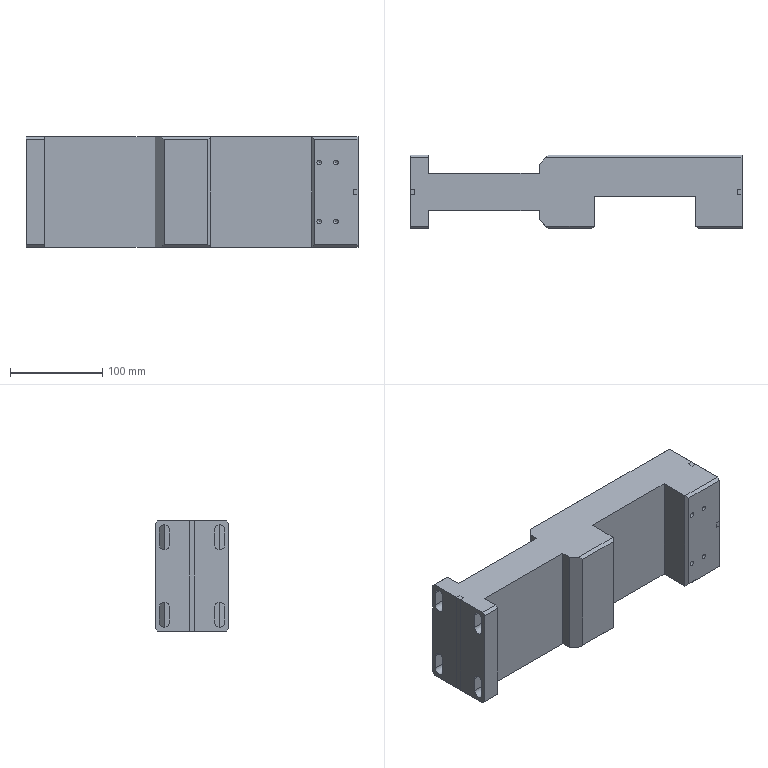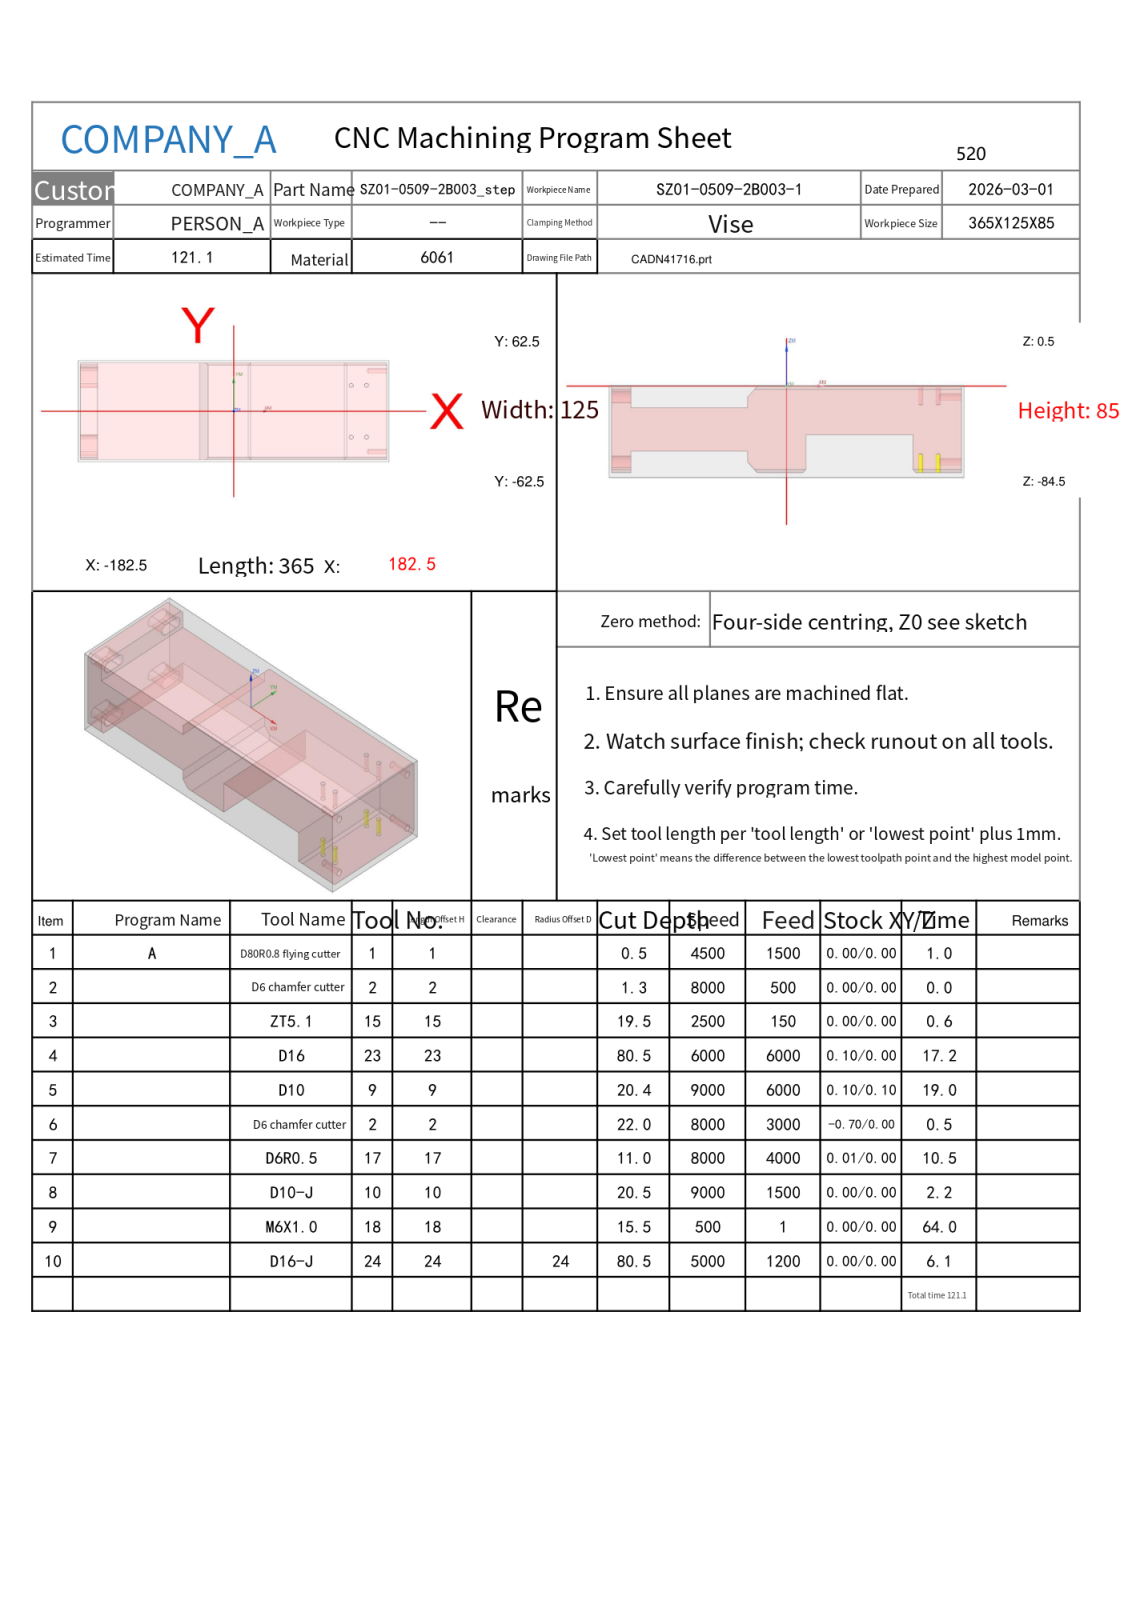NC program | NX | posted by the shop | part box 360 x 80 x 120 mm
Lines 904 to 4545 of 6444, first 3579 of 3642 lines:
N5 T09 M06
(D10  D=10. R=0. H=09 ce=0.10 di=0.10)
G00 G90 G54 X-98.6 Y6.407 M03 S9000
G43 H09 Z50.
M08
Z.5
G01 Y7.5 Z.471 F6000.
X-101.4 Z.398
Y-7.5 Z.005
X-98.6 Z-.068
Y7.5 Z-.461
X-100. Z-.498
X-101.4
Y-7.5
X-98.6
Y7.5
X-100.
Y12.
X-105.9
Y-12.
X-94.1
Y12.
X-100.
Y19.
X-112.9
Y-19.
X-87.1
Y19.
X-100.
Y26.
X-119.9
Y-26.
X-80.1
Y26.
X-100.
Y33.
X-126.9
Y-33.
X-73.1
Y33.
X-100.
Y40.
X-133.9
Y-40.
X-66.1
Y40.
X-100.
Y47.
X-140.9
Y-47.
X-59.1
Y47.
X-100.
Y54.
X-147.9
Y-54.
X-52.1
Y54.
X-100.
Y61.
X-154.9
Y-61.
X-45.1
Y61.
X-100.
X-100.5
Z.003
G00 Z.5
X-98.6 Y6.407
Z.003
G01 Y7.5 Z-.026
X-101.4 Z-.099
Y-7.5 Z-.492
X-98.6 Z-.566
Y7.5 Z-.958
X-100. Z-.995
X-101.4
Y-7.5
X-98.6
Y7.5
X-100.
Y12.
X-105.9
Y-12.
X-94.1
Y12.
X-100.
Y19.
X-112.9
Y-19.
X-87.1
Y19.
X-100.
Y26.
X-119.9
Y-26.
X-80.1
Y26.
X-100.
Y33.
X-126.9
Y-33.
X-73.1
Y33.
X-100.
Y40.
X-133.9
Y-40.
X-66.1
Y40.
X-100.
Y47.
X-140.9
Y-47.
X-59.1
Y47.
X-100.
Y54.
X-147.9
Y-54.
X-52.1
Y54.
X-100.
Y61.
X-154.9
Y-61.
X-45.1
Y61.
X-100.
X-100.5
Z-.495
G00 Z.003
X-98.6 Y6.407
Z-.495
G01 Y7.5 Z-.524
X-101.4 Z-.597
Y-7.5 Z-.99
X-98.6 Z-1.063
Y7.5 Z-1.456
X-100. Z-1.493
X-101.4
Y-7.5
X-98.6
Y7.5
X-100.
Y12.
X-105.9
Y-12.
X-94.1
Y12.
X-100.
Y19.
X-112.9
Y-19.
X-87.1
Y19.
X-100.
Y26.
X-119.9
Y-26.
X-80.1
Y26.
X-100.
Y33.
X-126.9
Y-33.
X-73.1
Y33.
X-100.
Y40.
X-133.9
Y-40.
X-66.1
Y40.
X-100.
Y47.
X-140.9
Y-47.
X-59.1
Y47.
X-100.
Y54.
X-147.9
Y-54.
X-52.1
Y54.
X-100.
Y61.
X-154.9
Y-61.
X-45.1
Y61.
X-100.
X-100.5
Z-.993
G00 Z-.495
X-98.6 Y6.407
Z-.993
G01 Y7.5 Z-1.021
X-101.4 Z-1.094
Y-7.5 Z-1.487
X-98.6 Z-1.561
Y7.5 Z-1.953
X-100. Z-1.99
X-101.4
Y-7.5
X-98.6
Y7.5
X-100.
Y12.
X-105.9
Y-12.
X-94.1
Y12.
X-100.
Y19.
X-112.9
Y-19.
X-87.1
Y19.
X-100.
Y26.
X-119.9
Y-26.
X-80.1
Y26.
X-100.
Y33.
X-126.9
Y-33.
X-73.1
Y33.
X-100.
Y40.
X-133.9
Y-40.
X-66.1
Y40.
X-100.
Y47.
X-140.9
Y-47.
X-59.1
Y47.
X-100.
Y54.
X-147.9
Y-54.
X-52.1
Y54.
X-100.
Y61.
X-154.9
Y-61.
X-45.1
Y61.
X-100.
X-100.5
Z-1.49
G00 Z-.993
X-98.6 Y6.407
Z-1.49
G01 Y7.5 Z-1.519
X-101.4 Z-1.592
Y-7.5 Z-1.985
X-98.6 Z-2.058
Y7.5 Z-2.451
X-100. Z-2.488
X-101.4
Y-7.5
X-98.6
Y7.5
X-100.
Y12.
X-105.9
Y-12.
X-94.1
Y12.
X-100.
Y19.
X-112.9
Y-19.
X-87.1
Y19.
X-100.
Y26.
X-119.9
Y-26.
X-80.1
Y26.
X-100.
Y33.
X-126.9
Y-33.
X-73.1
Y33.
X-100.
Y40.
X-133.9
Y-40.
X-66.1
Y40.
X-100.
Y47.
X-140.9
Y-47.
X-59.1
Y47.
X-100.
Y54.
X-147.9
Y-54.
X-52.1
Y54.
X-100.
Y61.
X-154.9
Y-61.
X-45.1
Y61.
X-100.
X-100.5
Z-1.988
G00 Z-1.49
X-98.6 Y6.407
Z-1.988
G01 Y7.5 Z-2.016
X-101.4 Z-2.089
Y-7.5 Z-2.482
X-98.6 Z-2.556
Y7.5 Z-2.948
X-100. Z-2.985
X-101.4
Y-7.5
X-98.6
Y7.5
X-100.
Y12.
X-105.9
Y-12.
X-94.1
Y12.
X-100.
Y19.
X-112.9
Y-19.
X-87.1
Y19.
X-100.
Y26.
X-119.9
Y-26.
X-80.1
Y26.
X-100.
Y33.
X-126.9
Y-33.
X-73.1
Y33.
X-100.
Y40.
X-133.9
Y-40.
X-66.1
Y40.
X-100.
Y47.
X-140.9
Y-47.
X-59.1
Y47.
X-100.
Y54.
X-147.9
Y-54.
X-52.1
Y54.
X-100.
Y61.
X-154.9
Y-61.
X-45.1
Y61.
X-100.
X-100.5
Z-2.485
G00 Z-1.988
X-98.6 Y6.407
Z-2.485
G01 Y7.5 Z-2.514
X-101.4 Z-2.587
Y-7.5 Z-2.98
X-98.6 Z-3.053
Y7.5 Z-3.446
X-100. Z-3.483
X-101.4
Y-7.5
X-98.6
Y7.5
X-100.
Y12.
X-105.9
Y-12.
X-94.1
Y12.
X-100.
Y19.
X-112.9
Y-19.
X-87.1
Y19.
X-100.
Y26.
X-119.9
Y-26.
X-80.1
Y26.
X-100.
Y33.
X-126.9
Y-33.
X-73.1
Y33.
X-100.
Y40.
X-133.9
Y-40.
X-66.1
Y40.
X-100.
Y47.
X-140.9
Y-47.
X-59.1
Y47.
X-100.
Y54.
X-147.9
Y-54.
X-52.1
Y54.
X-100.
Y61.
X-154.9
Y-61.
X-45.1
Y61.
X-100.
X-100.5
Z-2.983
G00 Z-2.485
X-98.6 Y6.407
Z-2.983
G01 Y7.5 Z-3.011
X-101.4 Z-3.084
Y-7.5 Z-3.477
X-98.6 Z-3.551
Y7.5 Z-3.943
X-100. Z-3.98
X-101.4
Y-7.5
X-98.6
Y7.5
X-100.
Y12.
X-105.9
Y-12.
X-94.1
Y12.
X-100.
Y19.
X-112.9
Y-19.
X-87.1
Y19.
X-100.
Y26.
X-119.9
Y-26.
X-80.1
Y26.
X-100.
Y33.
X-126.9
Y-33.
X-73.1
Y33.
X-100.
Y40.
X-133.9
Y-40.
X-66.1
Y40.
X-100.
Y47.
X-140.9
Y-47.
X-59.1
Y47.
X-100.
Y54.
X-147.9
Y-54.
X-52.1
Y54.
X-100.
Y61.
X-154.9
Y-61.
X-45.1
Y61.
X-100.
X-100.5
Z-3.48
G00 Z-2.983
X-98.6 Y6.407
Z-3.48
G01 Y7.5 Z-3.509
X-101.4 Z-3.582
Y-7.5 Z-3.975
X-98.6 Z-4.048
Y7.5 Z-4.441
X-100. Z-4.478
X-101.4
Y-7.5
X-98.6
Y7.5
X-100.
Y12.
X-105.9
Y-12.
X-94.1
Y12.
X-100.
Y19.
X-112.9
Y-19.
X-87.1
Y19.
X-100.
Y26.
X-119.9
Y-26.
X-80.1
Y26.
X-100.
Y33.
X-126.9
Y-33.
X-73.1
Y33.
X-100.
Y40.
X-133.9
Y-40.
X-66.1
Y40.
X-100.
Y47.
X-140.9
Y-47.
X-59.1
Y47.
X-100.
Y54.
X-147.9
Y-54.
X-52.1
Y54.
X-100.
Y61.
X-154.9
Y-61.
X-45.1
Y61.
X-100.
X-100.5
Z-3.978
G00 Z-3.48
X-98.6 Y6.407
Z-3.978
G01 Y7.5 Z-4.006
X-101.4 Z-4.079
Y-7.5 Z-4.472
X-98.6 Z-4.546
Y7.5 Z-4.938
X-100. Z-4.975
X-101.4
Y-7.5
X-98.6
Y7.5
X-100.
Y12.
X-105.9
Y-12.
X-94.1
Y12.
X-100.
Y19.
X-112.9
Y-19.
X-87.1
Y19.
X-100.
Y26.
X-119.9
Y-26.
X-80.1
Y26.
X-100.
Y33.
X-126.9
Y-33.
X-73.1
Y33.
X-100.
Y40.
X-133.9
Y-40.
X-66.1
Y40.
X-100.
Y47.
X-140.9
Y-47.
X-59.1
Y47.
X-100.
Y54.
X-147.9
Y-54.
X-52.1
Y54.
X-100.
Y61.
X-154.9
Y-61.
X-45.1
Y61.
X-100.
X-100.5
Z-4.475
G00 Z-3.978
X-98.6 Y6.407
Z-4.475
G01 Y7.5 Z-4.504
X-101.4 Z-4.577
Y-7.5 Z-4.97
X-98.6 Z-5.043
Y7.5 Z-5.436
X-100. Z-5.473
X-101.4
Y-7.5
X-98.6
Y7.5
X-100.
Y12.
X-105.9
Y-12.
X-94.1
Y12.
X-100.
Y19.
X-112.9
Y-19.
X-87.1
Y19.
X-100.
Y26.
X-119.9
Y-26.
X-80.1
Y26.
X-100.
Y33.
X-126.9
Y-33.
X-73.1
Y33.
X-100.
Y40.
X-133.9
Y-40.
X-66.1
Y40.
X-100.
Y47.
X-140.9
Y-47.
X-59.1
Y47.
X-100.
Y54.
X-147.9
Y-54.
X-52.1
Y54.
X-100.
Y61.
X-154.9
Y-61.
X-45.1
Y61.
X-100.
X-100.5
Z-4.973
G00 Z-4.475
X-98.6 Y6.407
Z-4.973
G01 Y7.5 Z-5.001
X-101.4 Z-5.074
Y-7.5 Z-5.467
X-98.6 Z-5.541
Y7.5 Z-5.933
X-100. Z-5.97
X-101.4
Y-7.5
X-98.6
Y7.5
X-100.
Y12.
X-105.9
Y-12.
X-94.1
Y12.
X-100.
Y19.
X-112.9
Y-19.
X-87.1
Y19.
X-100.
Y26.
X-119.9
Y-26.
X-80.1
Y26.
X-100.
Y33.
X-126.9
Y-33.
X-73.1
Y33.
X-100.
Y40.
X-133.9
Y-40.
X-66.1
Y40.
X-100.
Y47.
X-140.9
Y-47.
X-59.1
Y47.
X-100.
Y54.
X-147.9
Y-54.
X-52.1
Y54.
X-100.
Y61.
X-154.9
Y-61.
X-45.1
Y61.
X-100.
X-100.5
Z-5.47
G00 Z-4.973
X-98.6 Y6.407
Z-5.47
G01 Y7.5 Z-5.499
X-101.4 Z-5.572
Y-7.5 Z-5.965
X-98.6 Z-6.038
Y7.5 Z-6.431
X-100. Z-6.468
X-101.4
Y-7.5
X-98.6
Y7.5
X-100.
Y12.
X-105.9
Y-12.
X-94.1
Y12.
X-100.
Y19.
X-112.9
Y-19.
X-87.1
Y19.
X-100.
Y26.
X-119.9
Y-26.
X-80.1
Y26.
X-100.
Y33.
X-126.9
Y-33.
X-73.1
Y33.
X-100.
Y40.
X-133.9
Y-40.
X-66.1
Y40.
X-100.
Y47.
X-140.9
Y-47.
X-59.1
Y47.
X-100.
Y54.
X-147.9
Y-54.
X-52.1
Y54.
X-100.
Y61.
X-154.9
Y-61.
X-45.1
Y61.
X-100.
X-100.5
Z-5.968
G00 Z-5.47
X-98.6 Y6.407
Z-5.968
G01 Y7.5 Z-5.996
X-101.4 Z-6.069
Y-7.5 Z-6.462
X-98.6 Z-6.536
Y7.5 Z-6.928
X-100. Z-6.965
X-101.4
Y-7.5
X-98.6
Y7.5
X-100.
Y12.
X-105.9
Y-12.
X-94.1
Y12.
X-100.
Y19.
X-112.9
Y-19.
X-87.1
Y19.
X-100.
Y26.
X-119.9
Y-26.
X-80.1
Y26.
X-100.
Y33.
X-126.9
Y-33.
X-73.1
Y33.
X-100.
Y40.
X-133.9
Y-40.
X-66.1
Y40.
X-100.
Y47.
X-140.9
Y-47.
X-59.1
Y47.
X-100.
Y54.
X-147.9
Y-54.
X-52.1
Y54.
X-100.
Y61.
X-154.9
Y-61.
X-45.1
Y61.
X-100.
X-100.5
Z-6.465
G00 Z-5.968
X-98.6 Y6.407
Z-6.465
G01 Y7.5 Z-6.494
X-101.4 Z-6.567
Y-7.5 Z-6.96
X-98.6 Z-7.033
Y7.5 Z-7.426
X-100. Z-7.463
X-101.4
Y-7.5
X-98.6
Y7.5
X-100.
Y12.
X-105.9
Y-12.
X-94.1
Y12.
X-100.
Y19.
X-112.9
Y-19.
X-87.1
Y19.
X-100.
Y26.
X-119.9
Y-26.
X-80.1
Y26.
X-100.
Y33.
X-126.9
Y-33.
X-73.1
Y33.
X-100.
Y40.
X-133.9
Y-40.
X-66.1
Y40.
X-100.
Y47.
X-140.9
Y-47.
X-59.1
Y47.
X-100.
Y54.
X-147.9
Y-54.
X-52.1
Y54.
X-100.
Y61.
X-154.9
Y-61.
X-45.1
Y61.
X-100.
X-100.5
Z-6.963
G00 Z-6.465
X-98.6 Y6.407
Z-6.963
G01 Y7.5 Z-6.991
X-101.4 Z-7.064
Y-7.5 Z-7.457
X-98.6 Z-7.531
Y7.5 Z-7.923
X-100. Z-7.96
X-101.4
Y-7.5
X-98.6
Y7.5
X-100.
Y12.
X-105.9
Y-12.
X-94.1
Y12.
X-100.
Y19.
X-112.9
Y-19.
X-87.1
Y19.
X-100.
Y26.
X-119.9
Y-26.
X-80.1
Y26.
X-100.
Y33.
X-126.9
Y-33.
X-73.1
Y33.
X-100.
Y40.
X-133.9
Y-40.
X-66.1
Y40.
X-100.
Y47.
X-140.9
Y-47.
X-59.1
Y47.
X-100.
Y54.
X-147.9
Y-54.
X-52.1
Y54.
X-100.
Y61.
X-154.9
Y-61.
X-45.1
Y61.
X-100.
X-100.5
Z-7.46
G00 Z-6.963
X-98.6 Y6.407
Z-7.46
G01 Y7.5 Z-7.489
X-101.4 Z-7.562
Y-7.5 Z-7.955
X-98.6 Z-8.028
Y7.5 Z-8.421
X-100. Z-8.458
X-101.4
Y-7.5
X-98.6
Y7.5
X-100.
Y12.
X-105.9
Y-12.
X-94.1
Y12.
X-100.
Y19.
X-112.9
Y-19.
X-87.1
Y19.
X-100.
Y26.
X-119.9
Y-26.
X-80.1
Y26.
X-100.
Y33.
X-126.9
Y-33.
X-73.1
Y33.
X-100.
Y40.
X-133.9
Y-40.
X-66.1
Y40.
X-100.
Y47.
X-140.9
Y-47.
X-59.1
Y47.
X-100.
Y54.
X-147.9
Y-54.
X-52.1
Y54.
X-100.
Y61.
X-154.9
Y-61.
X-45.1
Y61.
X-100.
X-100.5
Z-7.958
G00 Z-7.46
X-98.6 Y6.407
Z-7.958
G01 Y7.5 Z-7.986
X-101.4 Z-8.059
Y-7.5 Z-8.452
X-98.6 Z-8.526
Y7.5 Z-8.918
X-100. Z-8.955
X-101.4
Y-7.5
X-98.6
Y7.5
X-100.
Y12.
X-105.9
Y-12.
X-94.1
Y12.
X-100.
Y19.
X-112.9
Y-19.
X-87.1
Y19.
X-100.
Y26.
X-119.9
Y-26.
X-80.1
Y26.
X-100.
Y33.
X-126.9
Y-33.
X-73.1
Y33.
X-100.
Y40.
X-133.9
Y-40.
X-66.1
Y40.
X-100.
Y47.
X-140.9
Y-47.
X-59.1
Y47.
X-100.
Y54.
X-147.9
Y-54.
X-52.1
Y54.
X-100.
Y61.
X-154.9
Y-61.
X-45.1
Y61.
X-100.
X-100.5
Z-8.455
G00 Z-7.958
X-98.6 Y6.407
Z-8.455
G01 Y7.5 Z-8.484
X-101.4 Z-8.557
Y-7.5 Z-8.95
X-98.6 Z-9.023
Y7.5 Z-9.416
X-100. Z-9.453
X-101.4
Y-7.5
X-98.6
Y7.5
X-100.
Y12.
X-105.9
Y-12.
X-94.1
Y12.
X-100.
Y19.
X-112.9
Y-19.
X-87.1
Y19.
X-100.
Y26.
X-119.9
Y-26.
X-80.1
Y26.
X-100.
Y33.
X-126.9
Y-33.
X-73.1
Y33.
X-100.
Y40.
X-133.9
Y-40.
X-66.1
Y40.
X-100.
Y47.
X-140.9
Y-47.
X-59.1
Y47.
X-100.
Y54.
X-147.9
Y-54.
X-52.1
Y54.
X-100.
Y61.
X-154.9
Y-61.
X-45.1
Y61.
X-100.
X-100.5
Z-8.953
G00 Z-8.455
X-98.6 Y6.407
Z-8.953
G01 Y7.5 Z-8.981
X-101.4 Z-9.054
Y-7.5 Z-9.447
X-98.6 Z-9.521
Y7.5 Z-9.913
X-100. Z-9.95
X-101.4
Y-7.5
X-98.6
Y7.5
X-100.
Y12.
X-105.9
Y-12.
X-94.1
Y12.
X-100.
Y19.
X-112.9
Y-19.
X-87.1
Y19.
X-100.
Y26.
X-119.9
Y-26.
X-80.1
Y26.
X-100.
Y33.
X-126.9
Y-33.
X-73.1
Y33.
X-100.
Y40.
X-133.9
Y-40.
X-66.1
Y40.
X-100.
Y47.
X-140.9
Y-47.
X-59.1
Y47.
X-100.
Y54.
X-147.9
Y-54.
X-52.1
Y54.
X-100.
Y61.
X-154.9
Y-61.
X-45.1
Y61.
X-100.
X-100.5
Z-9.45
G00 Z-8.953
X-98.6 Y6.407
Z-9.45
G01 Y7.5 Z-9.479
X-101.4 Z-9.552
Y-7.5 Z-9.945
X-98.6 Z-10.018
Y7.5 Z-10.411
X-100. Z-10.448
X-101.4
Y-7.5
X-98.6
Y7.5
X-100.
Y12.
X-105.9
Y-12.
X-94.1
Y12.
X-100.
Y19.
X-112.9
Y-19.
X-87.1
Y19.
X-100.
Y26.
X-119.9
Y-26.
X-80.1
Y26.
X-100.
Y33.
X-126.9
Y-33.
X-73.1
Y33.
X-100.
Y40.
X-133.9
Y-40.
X-66.1
Y40.
X-100.
Y47.
X-140.9
Y-47.
X-59.1
Y47.
X-100.
Y54.
X-147.9
Y-54.
X-52.1
Y54.
X-100.
Y61.
X-154.9
Y-61.
X-45.1
Y61.
X-100.
X-100.5
Z-9.948
G00 Z-9.45
X-98.6 Y6.407
Z-9.948
G01 Y7.5 Z-9.976
X-101.4 Z-10.049
Y-7.5 Z-10.442
X-98.6 Z-10.516
Y7.5 Z-10.908
X-100. Z-10.945
X-101.4
Y-7.5
X-98.6
Y7.5
X-100.
Y12.
X-105.9
Y-12.
X-94.1
Y12.
X-100.
Y19.
X-112.9
Y-19.
X-87.1
Y19.
X-100.
Y26.
X-119.9
Y-26.
X-80.1
Y26.
X-100.
Y33.
X-126.9
Y-33.
X-73.1
Y33.
X-100.
Y40.
X-133.9
Y-40.
X-66.1
Y40.
X-100.
Y47.
X-140.9
Y-47.
X-59.1
Y47.
X-100.
Y54.
X-147.9
Y-54.
X-52.1
Y54.
X-100.
Y61.
X-154.9
Y-61.
X-45.1
Y61.
X-100.
X-100.5
Z-10.445
G00 Z-9.948
X-98.6 Y6.407
Z-10.445
G01 Y7.5 Z-10.474
X-101.4 Z-10.547
Y-7.5 Z-10.94
X-98.6 Z-11.013
Y7.5 Z-11.406
X-100. Z-11.443
X-101.4
Y-7.5
X-98.6
Y7.5
X-100.
Y12.
X-105.9
Y-12.
X-94.1
Y12.
X-100.
Y19.
X-112.9
Y-19.
X-87.1
Y19.
X-100.
Y26.
X-119.9
Y-26.
X-80.1
Y26.
X-100.
Y33.
X-126.9
Y-33.
X-73.1
Y33.
X-100.
Y40.
X-133.9
Y-40.
X-66.1
Y40.
X-100.
Y47.
X-140.9
Y-47.
X-59.1
Y47.
X-100.
Y54.
X-147.9
Y-54.
X-52.1
Y54.
X-100.
Y61.
X-154.9
Y-61.
X-45.1
Y61.
X-100.
X-100.5
Z-10.943
G00 Z-10.445
X-98.6 Y6.407
Z-10.943
G01 Y7.5 Z-10.971
X-101.4 Z-11.044
Y-7.5 Z-11.437
X-98.6 Z-11.511
Y7.5 Z-11.903
X-100. Z-11.94
X-101.4
Y-7.5
X-98.6
Y7.5
X-100.
Y12.
X-105.9
Y-12.
X-94.1
Y12.
X-100.
Y19.
X-112.9
Y-19.
X-87.1
Y19.
X-100.
Y26.
X-119.9
Y-26.
X-80.1
Y26.
X-100.
Y33.
X-126.9
Y-33.
X-73.1
Y33.
X-100.
Y40.
X-133.9
Y-40.
X-66.1
Y40.
X-100.
Y47.
X-140.9
Y-47.
X-59.1
Y47.
X-100.
Y54.
X-147.9
Y-54.
X-52.1
Y54.
X-100.
Y61.
X-154.9
Y-61.
X-45.1
Y61.
X-100.
X-100.5
Z-11.44
G00 Z-10.943
X-98.6 Y6.407
Z-11.44
G01 Y7.5 Z-11.469
X-101.4 Z-11.542
Y-7.5 Z-11.935
X-98.6 Z-12.008
Y7.5 Z-12.401
X-100. Z-12.438
X-101.4
Y-7.5
X-98.6
Y7.5
X-100.
Y12.
X-105.9
Y-12.
X-94.1
Y12.
X-100.
Y19.
X-112.9
Y-19.
X-87.1
Y19.
X-100.
Y26.
X-119.9
Y-26.
X-80.1
Y26.
X-100.
Y33.
X-126.9
Y-33.
X-73.1
Y33.
X-100.
Y40.
X-133.9
Y-40.
X-66.1
Y40.
X-100.
Y47.
X-140.9
Y-47.
X-59.1
Y47.
X-100.
Y54.
X-147.9
Y-54.
X-52.1
Y54.
X-100.
Y61.
X-154.9
Y-61.
X-45.1
Y61.
X-100.
X-100.5
Z-11.938
G00 Z-11.44
X-98.6 Y6.407
Z-11.938
G01 Y7.5 Z-11.966
X-101.4 Z-12.039
Y-7.5 Z-12.432
X-98.6 Z-12.506
Y7.5 Z-12.898
X-100. Z-12.935
X-101.4
Y-7.5
X-98.6
Y7.5
X-100.
Y12.
X-105.9
Y-12.
X-94.1
Y12.
X-100.
Y19.
X-112.9
Y-19.
X-87.1
Y19.
X-100.
Y26.
X-119.9
Y-26.
X-80.1
Y26.
X-100.
Y33.
X-126.9
Y-33.
X-73.1
Y33.
X-100.
Y40.
X-133.9
Y-40.
X-66.1
Y40.
X-100.
Y47.
X-140.9
Y-47.
X-59.1
Y47.
X-100.
Y54.
X-147.9
Y-54.
X-52.1
Y54.
X-100.
Y61.
X-154.9
Y-61.
X-45.1
Y61.
X-100.
X-100.5
Z-12.435
G00 Z-11.938
X-98.6 Y6.407
Z-12.435
G01 Y7.5 Z-12.464
X-101.4 Z-12.537
Y-7.5 Z-12.93
X-98.6 Z-13.003
Y7.5 Z-13.396
X-100. Z-13.433
X-101.4
Y-7.5
X-98.6
Y7.5
X-100.
Y12.
X-105.9
Y-12.
X-94.1
Y12.
X-100.
Y19.
X-112.9
Y-19.
X-87.1
Y19.
X-100.
Y26.
X-119.9
Y-26.
X-80.1
Y26.
X-100.
Y33.
X-126.9
Y-33.
X-73.1
Y33.
X-100.
Y40.
X-133.9
Y-40.
X-66.1
Y40.
X-100.
Y47.
X-140.9
Y-47.
X-59.1
Y47.
X-100.
Y54.
X-147.9
Y-54.
X-52.1
Y54.
X-100.
Y61.
X-154.9
Y-61.
X-45.1
Y61.
X-100.
X-100.5
Z-12.933
G00 Z-12.435
X-98.6 Y6.407
Z-12.933
G01 Y7.5 Z-12.961
X-101.4 Z-13.034
Y-7.5 Z-13.427
X-98.6 Z-13.501
Y7.5 Z-13.893
X-100. Z-13.93
X-101.4
Y-7.5
X-98.6
Y7.5
X-100.
Y12.
X-105.9
Y-12.
X-94.1
Y12.
X-100.
Y19.
X-112.9
Y-19.
X-87.1
Y19.
X-100.
Y26.
X-119.9
Y-26.
X-80.1
Y26.
X-100.
Y33.
X-126.9
Y-33.
X-73.1
Y33.
X-100.
Y40.
X-133.9
Y-40.
X-66.1
Y40.
X-100.
Y47.
X-140.9
Y-47.
X-59.1
Y47.
X-100.
Y54.
X-147.9
Y-54.
X-52.1
Y54.
X-100.
Y61.
X-154.9
Y-61.
X-45.1
Y61.
X-100.
X-100.5
Z-13.43
G00 Z-12.933
X-98.6 Y6.407
Z-13.43
G01 Y7.5 Z-13.459
X-101.4 Z-13.532
Y-7.5 Z-13.925
X-98.6 Z-13.998
Y7.5 Z-14.391
X-100. Z-14.428
X-101.4
Y-7.5
X-98.6
Y7.5
X-100.
Y12.
X-105.9
Y-12.
X-94.1
Y12.
X-100.
Y19.
X-112.9
Y-19.
X-87.1
Y19.
X-100.
Y26.
X-119.9
Y-26.
X-80.1
Y26.
X-100.
Y33.
X-126.9
Y-33.
X-73.1
Y33.
X-100.
Y40.
X-133.9
Y-40.
X-66.1
Y40.
X-100.
Y47.
X-140.9
Y-47.
X-59.1
Y47.
X-100.
Y54.
X-147.9
Y-54.
X-52.1
Y54.
X-100.
Y61.
X-154.9
Y-61.
X-45.1
Y61.
X-100.
X-100.5
Z-13.928
G00 Z-13.43
X-98.6 Y6.407
Z-13.928
G01 Y7.5 Z-13.956
X-101.4 Z-14.029
Y-7.5 Z-14.422
X-98.6 Z-14.496
Y7.5 Z-14.888
X-100. Z-14.925
X-101.4
Y-7.5
X-98.6
Y7.5
X-100.
Y12.
X-105.9
Y-12.
X-94.1
Y12.
X-100.
Y19.
X-112.9
Y-19.
X-87.1
Y19.
X-100.
Y26.
X-119.9
Y-26.
X-80.1
Y26.
X-100.
Y33.
X-126.9
Y-33.
X-73.1
Y33.
X-100.
Y40.
X-133.9
Y-40.
X-66.1
Y40.
X-100.
Y47.
X-140.9
Y-47.
X-59.1
Y47.
X-100.
Y54.
X-147.9
Y-54.
X-52.1
Y54.
X-100.
Y61.
X-154.9
Y-61.
X-45.1
Y61.
X-100.
X-100.5
Z-14.425
G00 Z-13.928
X-98.6 Y6.407
Z-14.425
G01 Y7.5 Z-14.454
X-101.4 Z-14.527
Y-7.5 Z-14.92
X-98.6 Z-14.993
Y7.5 Z-15.386
X-100. Z-15.423
X-101.4
Y-7.5
X-98.6
Y7.5
X-100.
Y12.
X-105.9
Y-12.
X-94.1
Y12.
X-100.
Y19.
X-112.9
Y-19.
X-87.1
Y19.
X-100.
Y26.
X-119.9
Y-26.
X-80.1
Y26.
X-100.
Y33.
X-126.9
Y-33.
X-73.1
Y33.
X-100.
Y40.
X-133.9
Y-40.
X-66.1
Y40.
X-100.
Y47.
X-140.9
Y-47.
X-59.1
Y47.
X-100.
Y54.
X-147.9
Y-54.
X-52.1
Y54.
X-100.
Y61.
X-154.9
Y-61.
X-45.1
Y61.
X-100.
X-100.5
Z-14.923
G00 Z-14.425
X-98.6 Y6.407
Z-14.923
G01 Y7.5 Z-14.951
X-101.4 Z-15.024
Y-7.5 Z-15.417
X-98.6 Z-15.491
Y7.5 Z-15.883
X-100. Z-15.92
X-101.4
Y-7.5
X-98.6
Y7.5
X-100.
Y12.
X-105.9
Y-12.
X-94.1
Y12.
X-100.
Y19.
X-112.9
Y-19.
X-87.1
Y19.
X-100.
Y26.
X-119.9
Y-26.
X-80.1
Y26.
X-100.
Y33.
X-126.9
Y-33.
X-73.1
Y33.
X-100.
Y40.
X-133.9
Y-40.
X-66.1
Y40.
X-100.
Y47.
X-140.9
Y-47.
X-59.1
Y47.
X-100.
Y54.
X-147.9
Y-54.
X-52.1
Y54.
X-100.
Y61.
X-154.9
Y-61.
X-45.1
Y61.
X-100.
X-100.5
Z-15.42
G00 Z-14.923
X-98.6 Y6.407
Z-15.42
G01 Y7.5 Z-15.449
X-101.4 Z-15.522
Y-7.5 Z-15.915
X-98.6 Z-15.988
Y7.5 Z-16.381
X-100. Z-16.418
X-101.4
Y-7.5
X-98.6
Y7.5
X-100.
Y12.
X-105.9
Y-12.
X-94.1
Y12.
X-100.
Y19.
X-112.9
Y-19.
X-87.1
Y19.
X-100.
Y26.
X-119.9
Y-26.
X-80.1
Y26.
X-100.
Y33.
X-126.9
Y-33.
X-73.1
Y33.
X-100.
Y40.
X-133.9
Y-40.
X-66.1
Y40.
X-100.
Y47.
X-140.9
Y-47.
X-59.1
Y47.
X-100.
Y54.
X-147.9
Y-54.
X-52.1
Y54.
X-100.
Y61.
X-154.9
Y-61.
X-45.1
Y61.
X-100.
X-100.5
Z-15.918
G00 Z-15.42
X-98.6 Y6.407
Z-15.918
G01 Y7.5 Z-15.946
X-101.4 Z-16.019
Y-7.5 Z-16.412
X-98.6 Z-16.486
Y7.5 Z-16.878
X-100. Z-16.915
X-101.4
Y-7.5
X-98.6
Y7.5
X-100.
Y12.
X-105.9
Y-12.
X-94.1
Y12.
X-100.
Y19.
X-112.9
Y-19.
X-87.1
Y19.
X-100.
Y26.
X-119.9
Y-26.
X-80.1
Y26.
X-100.
Y33.
X-126.9
Y-33.
X-73.1
Y33.
X-100.
Y40.
X-133.9
Y-40.
X-66.1
Y40.
X-100.
Y47.
X-140.9
Y-47.
X-59.1
Y47.
X-100.
Y54.
X-147.9
Y-54.
X-52.1
Y54.
X-100.
Y61.
X-154.9
Y-61.
X-45.1
Y61.
X-100.
X-100.5
Z-16.415
G00 Z-15.918
X-98.6 Y6.407
Z-16.415
G01 Y7.5 Z-16.444
X-101.4 Z-16.517
Y-7.5 Z-16.91
X-98.6 Z-16.983
Y7.5 Z-17.376
X-100. Z-17.413
X-101.4
Y-7.5
X-98.6
Y7.5
X-100.
Y12.
X-105.9
Y-12.
X-94.1
Y12.
X-100.
Y19.
X-112.9
Y-19.
X-87.1
Y19.
X-100.
Y26.
X-119.9
Y-26.
X-80.1
Y26.
X-100.
Y33.
X-126.9
Y-33.
X-73.1
Y33.
X-100.
Y40.
X-133.9
Y-40.
X-66.1
Y40.
X-100.
Y47.
X-140.9
Y-47.
X-59.1
Y47.
X-100.
Y54.
X-147.9
Y-54.
X-52.1
Y54.
X-100.
Y61.
X-154.9
Y-61.
X-45.1
Y61.
X-100.
X-100.5
Z-16.913
G00 Z-16.415
X-98.6 Y6.407
Z-16.913
G01 Y7.5 Z-16.941
X-101.4 Z-17.014
Y-7.5 Z-17.407
X-98.6 Z-17.481
Y7.5 Z-17.873
X-100. Z-17.91
X-101.4
Y-7.5
X-98.6
Y7.5
X-100.
Y12.
X-105.9
Y-12.
X-94.1
Y12.
X-100.
Y19.
X-112.9
Y-19.
X-87.1
Y19.
X-100.
Y26.
X-119.9
Y-26.
X-80.1
Y26.
X-100.
Y33.
X-126.9
Y-33.
X-73.1
Y33.
X-100.
Y40.
X-133.9
Y-40.
X-66.1
Y40.
X-100.
Y47.
X-140.9
Y-47.
X-59.1
Y47.
X-100.
Y54.
X-147.9
Y-54.
X-52.1
Y54.
X-100.
Y61.
X-154.9
Y-61.
X-45.1
Y61.
X-100.
X-100.5
Z-17.41
G00 Z-16.913
X-98.6 Y6.407
Z-17.41
G01 Y7.5 Z-17.439
X-101.4 Z-17.512
Y-7.5 Z-17.905
X-98.6 Z-17.978
Y7.5 Z-18.371
X-100. Z-18.408
X-101.4
Y-7.5
X-98.6
Y7.5
X-100.
Y12.
X-105.9
Y-12.
X-94.1
Y12.
X-100.
Y19.
X-112.9
Y-19.
X-87.1
Y19.
X-100.
Y26.
X-119.9
Y-26.
X-80.1
Y26.
X-100.
Y33.
X-126.9
Y-33.
X-73.1
Y33.
X-100.
Y40.
X-133.9
Y-40.
X-66.1
Y40.
X-100.
Y47.
X-140.9
Y-47.
X-59.1
Y47.
X-100.
Y54.
X-147.9
Y-54.
X-52.1
Y54.
X-100.
Y61.
X-154.9
Y-61.
X-45.1
Y61.
X-100.
X-100.5
Z-17.908
G00 Z-17.41
X-98.6 Y6.407
Z-17.908
G01 Y7.5 Z-17.936
X-101.4 Z-18.009
Y-7.5 Z-18.402
X-98.6 Z-18.476
Y7.5 Z-18.868
X-100. Z-18.905
X-101.4
Y-7.5
X-98.6
Y7.5
X-100.
Y12.
X-105.9
Y-12.
X-94.1
Y12.
X-100.
Y19.
X-112.9
Y-19.
X-87.1
Y19.
X-100.
Y26.
X-119.9
Y-26.
X-80.1
Y26.
X-100.
Y33.
X-126.9
Y-33.
X-73.1
Y33.
X-100.
Y40.
X-133.9
Y-40.
X-66.1
Y40.
X-100.
Y47.
X-140.9
Y-47.
X-59.1
Y47.
X-100.
Y54.
X-147.9
Y-54.
X-52.1
Y54.
X-100.
Y61.
X-154.9
Y-61.
X-45.1
Y61.
X-100.
X-100.5
Z-18.405
G00 Z-17.908
X-98.6 Y6.407
Z-18.405
G01 Y7.5 Z-18.434
X-101.4 Z-18.507
Y-7.5 Z-18.9
X-98.6 Z-18.973
Y7.5 Z-19.366
X-100. Z-19.403
X-101.4
Y-7.5
X-98.6
Y7.5
X-100.
Y12.
X-105.9
Y-12.
X-94.1
Y12.
X-100.
Y19.
X-112.9
Y-19.
X-87.1
Y19.
X-100.
Y26.
X-119.9
Y-26.
X-80.1
Y26.
X-100.
Y33.
X-126.9
Y-33.
X-73.1
Y33.
X-100.
Y40.
X-133.9
Y-40.
X-66.1
Y40.
X-100.
Y47.
X-140.9
Y-47.
X-59.1
Y47.
X-100.
Y54.
X-147.9
Y-54.
X-52.1
Y54.
X-100.
Y61.
X-154.9
Y-61.
X-45.1
Y61.
X-100.
X-100.5
Z-18.903
G00 Z-18.405
X-98.6 Y6.407
Z-18.903
G01 Y7.5 Z-18.931
X-101.4 Z-19.004
Y-7.5 Z-19.397
X-98.6 Z-19.471
Y7.5 Z-19.863
X-100. Z-19.9
X-101.4
Y-7.5
X-98.6
Y7.5
X-100.
Y12.
X-105.9
Y-12.
X-94.1
Y12.
X-100.
Y19.
X-112.9
Y-19.
X-87.1
Y19.
X-100.
Y26.
X-119.9
Y-26.
X-80.1
Y26.
X-100.
Y33.
X-126.9
Y-33.
X-73.1
Y33.
X-100.
Y40.
X-133.9
Y-40.
X-66.1
Y40.
X-100.
Y47.
X-140.9
Y-47.
X-59.1
Y47.
X-100.
Y54.
X-147.9
Y-54.
X-52.1
Y54.
X-100.
Y61.
X-154.9
Y-61.
X-45.1
Y61.
X-100.
X-100.5
Z-19.4
G00 Z50.
G00 G90 X-33.344 Y-74.5 M03 S8000
Z10.5
Z.8
G01 Z-.4 F4000.
X-33.345 Y-67.08
G03 X-40.345 Y-60.08 I-7. J0.0
G01 X-45.069
X-45.154 Y-60.085
X-45.149 Y-60.
Y60.
X-45.154 Y60.085
X-45.069 Y60.08
X-38.071
X-38.014 Y60.056
X-35.54 Y57.582
X-35.541 Y55.58
Y-55.58
X-35.54 Y-57.582
X-37.39 Y-59.432
G02 X-37.885 Y-59.637 I-.495 J.495
X-38.51 Y-59.251 I0.0 J.7
G01 X-40.187 Y-55.906
G03 X-40.517 Y-55.528 I-.894 J-.449
G02 X-40.649 Y-55.281 I.169 J.248
G01 Y55.281
G02 X-40.349 Y55.58 I.3 J-.001
G01 X-40.34
G02 X-40.041 Y55.281 I-.001 J-.3
G01 Y-55.281
G02 X-40.341 Y-55.58 I-.3 J.001
G01 X-40.345
X-40.35
G02 X-40.65 Y-55.279 I.001 J.301
G01 X-40.649 Y-55.255
G03 X-47.649 Y-48.255 I-7. J0.0
G01 Z.8
G00 Z3.
G01 X-33.344 Y-74.5 F6000.
G00 Z.4
G01 Z-.8 F4000.
X-33.345 Y-67.08
G03 X-40.345 Y-60.08 I-7. J0.0
G01 X-45.069
X-45.154 Y-60.085
X-45.149 Y-60.
Y60.
X-45.154 Y60.085
X-45.069 Y60.08
X-38.071
X-38.014 Y60.056
X-35.94 Y57.982
Y-57.982
X-38.014 Y-60.056
X-38.071 Y-60.08
X-40.345
X-40.845
G03 X-47.845 Y-67.08 I0.0 J-7.
G01 X-47.844 Y-74.5
Z.4
G00 Z2.6
G01 X-33.344 F6000.
G00 Z0.0
G01 Z-1.2 F4000.
X-33.345 Y-67.08
G03 X-40.345 Y-60.08 I-7. J0.0
G01 X-45.069
X-45.154 Y-60.085
X-45.149 Y-60.
Y60.
X-45.154 Y60.085
X-45.069 Y60.08
X-38.071
X-38.014 Y60.056
X-36.34 Y58.382
Y-58.382
X-38.014 Y-60.056
X-38.071 Y-60.08
X-40.345
X-40.845
G03 X-47.845 Y-67.08 I0.0 J-7.
G01 X-47.844 Y-74.5
Z0.0
G00 Z2.2
G01 X-33.344 F6000.
G00 Z-.4
G01 Z-1.6 F4000.
X-33.345 Y-67.08
G03 X-40.345 Y-60.08 I-7. J0.0
G01 X-45.069
X-45.154 Y-60.085
X-45.149 Y-60.
Y60.
X-45.154 Y60.085
X-45.069 Y60.08
X-38.071
X-38.014 Y60.056
X-36.74 Y58.782
Y-58.782
X-38.014 Y-60.056
X-38.071 Y-60.08
X-40.345
X-40.845
G03 X-47.845 Y-67.08 I0.0 J-7.
G01 X-47.844 Y-74.5
Z-.4
G00 Z1.8
G01 X-36.844 F6000.
G00 Z-.8
G01 Z-2. F4000.
X-36.845 Y-63.58
G03 X-40.345 Y-60.08 I-3.5 J0.0
G01 X-45.069
X-45.154 Y-60.085
X-45.149 Y-60.
Y60.
X-45.154 Y60.085
X-45.069 Y60.08
X-38.071
X-38.014 Y60.056
X-37.14 Y59.182
Y-59.182
X-38.014 Y-60.056
X-38.071 Y-60.08
X-40.345
X-40.845
G03 X-47.845 Y-67.08 I0.0 J-7.
G01 X-47.844 Y-74.5
Z-.8
G00 Z1.4
G01 X-36.844 F6000.
G00 Z-1.2
G01 Z-2.4 F4000.
X-36.845 Y-63.58
G03 X-40.345 Y-60.08 I-3.5 J0.0
G01 X-45.069
X-45.154 Y-60.085
X-45.149 Y-60.
Y60.
X-45.154 Y60.085
X-45.069 Y60.08
X-38.071
X-38.014 Y60.056
X-37.54 Y59.582
Y-59.582
X-38.014 Y-60.056
X-38.071 Y-60.08
X-40.345
X-40.845
G03 X-47.845 Y-67.08 I0.0 J-7.
G01 X-47.844 Y-74.5
Z-1.2
G00 Z1.
G01 X-37.87 F6000.
G00 Z-1.6
G01 Z-2.8 F4000.
Y-61.105
G03 X-40.345 Y-60.08 I-2.475 J-2.475
G01 X-45.069
X-45.154 Y-60.085
X-45.149 Y-60.
Y60.
X-45.154 Y60.085
X-45.069 Y60.08
X-38.071
X-38.014 Y60.056
X-37.94 Y59.982
Y-59.982
X-38.014 Y-60.056
X-38.071 Y-60.08
X-40.345
X-40.845
G03 X-47.845 Y-67.08 I0.0 J-7.
G01 X-47.844 Y-74.5
Z-1.6
G00 Z.6
G01 X-39.32 F6000.
G00 Z-2.
G01 Z-3.2 F4000.
Y-57.605
G03 X-40.345 Y-60.08 I2.475 J-2.475
G01 X-45.069
X-45.154 Y-60.085
X-45.149 Y-60.
Y60.
X-45.154 Y60.085
X-45.069 Y60.08
X-38.34
Y-60.08
X-40.345
X-40.845
G03 X-47.845 Y-67.08 I0.0 J-7.
G01 X-47.844 Y-74.5
Z-2.
G00 Z.2
G01 X-39.32 F6000.
G00 Z-2.4
G01 Z-3.6 F4000.
Y-57.605
G03 X-40.345 Y-60.08 I2.475 J-2.475
G01 X-45.069
X-45.154 Y-60.085
X-45.149 Y-60.
Y60.
X-45.154 Y60.085
X-45.069 Y60.08
X-38.74
Y-60.08
X-40.345
X-40.845
G03 X-47.845 Y-67.08 I0.0 J-7.
G01 X-47.844 Y-74.5
Z-2.4
G00 Z-.2
G01 X-39.32 F6000.
G00 Z-2.8
G01 Z-4. F4000.
Y-57.605
G03 X-40.345 Y-60.08 I2.475 J-2.475
G01 X-45.069
X-45.154 Y-60.085
X-45.149 Y-60.
Y60.
X-45.154 Y60.085
X-45.069 Y60.08
X-39.14
Y-60.08
X-40.345
X-40.845
G03 X-47.845 Y-67.08 I0.0 J-7.
G01 X-47.844 Y-74.5
Z-2.8
G00 Z-.6
G01 X-49.604 F6000.
G00 Z-3.2
G01 Z-4.4 F4000.
X-42.372 Y-69.77
G03 X-39.203 Y-63.911 I-3.832 J5.858
X-40.345 Y-60.08 I-7. J0.0
G01 X-45.069
X-45.154 Y-60.085
X-45.149 Y-60.
Y60.
X-45.154 Y60.085
X-45.069 Y60.08
X-39.53
Y-60.08
X-40.345
X-40.845
G03 X-47.845 Y-67.08 I0.0 J-7.
G01 X-47.844 Y-74.5
Z-3.2
G00 Z-1.
G01 X-40.345 F6000.
G00 Z-3.6
G01 Z-4.8 F4000.
Y-60.08
X-45.069
X-45.154 Y-60.085
X-45.149 Y-60.
Y60.
X-45.154 Y60.085
X-45.069 Y60.08
X-39.94
Y-60.08
X-40.345
X-40.845
G03 X-47.845 Y-67.08 I0.0 J-7.
G01 X-47.844 Y-74.5
Z-3.6
G00 Z-1.4
G01 X-40.345 F6000.
G00 Z-4.
G01 Z-5.2 F4000.
Y-60.08
X-45.069
X-45.154 Y-60.085
X-45.149 Y-60.
Y60.
X-45.154 Y60.085
X-45.069 Y60.08
X-40.34
Y-60.08
X-40.345
X-40.34
X-40.341 Y-59.585
G03 X-47.341 Y-52.585 I-7. J0.0
G01 Z-4.
G00 Z3.
G01 X-47.539 Y-74.5 F6000.
G00 Z-4.4
G01 Z-5.6 F4000.
Y-67.275
G03 X-40.737 Y-60.277 I-.198 J6.997
G01 X-40.74 Y-60.08
X-45.069
X-45.154 Y-60.085
X-45.149 Y-60.
Y60.
X-45.154 Y60.085
X-45.069 Y60.08
X-40.74
Y-60.08
X-41.24
G03 X-48.24 Y-67.08 I0.0 J-7.
G01 X-48.239 Y-74.5
Z-4.4
G00 Z-2.2
G01 X-42.079 F6000.
G00 Z-4.8
G01 Z-6. F4000.
Y-57.605
G03 X-43.105 Y-60.08 I2.475 J-2.475
G01 X-45.069
X-45.154 Y-60.085
X-45.149 Y-60.
Y60.
X-45.154 Y60.085
X-45.069 Y60.08
X-41.14
Y-60.08
X-43.105
X-43.605
G03 X-50.604 Y-67.08 I0.0 J-7.
G01 Y-74.5
Z-4.8
G00 Z-2.6
G01 X-42.079 F6000.
G00 Z-5.2
G01 Z-6.4 F4000.
Y-57.605
G03 X-43.105 Y-60.08 I2.475 J-2.475
G01 X-45.069
X-45.154 Y-60.085
X-45.149 Y-60.
Y60.
X-45.154 Y60.085
X-45.069 Y60.08
X-41.54
Y-60.08
X-43.105
X-43.605
G03 X-50.604 Y-67.08 I0.0 J-7.
G01 Y-74.5
Z-5.2
G00 Z-3.
G01 X-42.079 F6000.
G00 Z-5.6
G01 Z-6.8 F4000.
Y-57.605
G03 X-43.105 Y-60.08 I2.475 J-2.475
G01 X-45.069
X-45.154 Y-60.085
X-45.149 Y-60.
Y60.
X-45.154 Y60.085
X-45.069 Y60.08
X-41.94
Y-60.08
X-43.105
X-43.605
G03 X-50.604 Y-67.08 I0.0 J-7.
G01 Y-74.5
Z-5.6
G00 Z-3.4
G01 X-52.125 F6000.
G00 Z-6.
G01 Z-7.2 F4000.
X-45.049 Y-69.786
G03 X-41.93 Y-63.961 I-3.881 J5.826
X-43.105 Y-60.08 I-7. J0.0
G01 X-45.069
X-45.154 Y-60.085
X-45.149 Y-60.
Y60.
X-45.154 Y60.085
X-45.069 Y60.08
X-42.34
Y-60.08
X-43.105
X-43.605
G03 X-50.604 Y-67.08 I0.0 J-7.
G01 Y-74.5
Z-6.
G00 Z-3.8
G01 X-43.105 F6000.
G00 Z-6.4
G01 Z-7.6 F4000.
Y-60.08
X-45.069
X-45.154 Y-60.085
X-45.149 Y-60.
Y60.
X-45.154 Y60.085
X-45.069 Y60.08
X-42.74
Y-60.08
X-43.105
X-43.605
G03 X-50.604 Y-67.08 I0.0 J-7.
G01 Y-74.5
Z-6.4
G00 Z-4.2
G01 X-49.952 F6000.
G00 Z-6.8
G01 Z-8. F4000.
Y-67.263
G03 X-43.137 Y-60.265 I-.185 J6.998
G01 X-43.14 Y-60.08
X-45.069
X-45.154 Y-60.085
X-45.149 Y-60.
Y60.
X-45.154 Y60.085
X-45.069 Y60.08
X-43.14
Y-60.08
X-43.64
G03 X-50.64 Y-67.08 I0.0 J-7.
G01 X-50.639 Y-74.5
Z-6.8
G00 Z-4.6
G01 X-53.367 F6000.
G00 Z-7.2
G01 Z-8.4 F4000.
X-46.264 Y-69.784
G03 X-43.136 Y-63.952 I-3.872 J5.831
X-44.305 Y-60.08 I-7. J0.0
G01 X-45.069
X-45.154 Y-60.085
X-45.149 Y-60.
Y60.
X-45.154 Y60.085
X-45.069 Y60.08
X-43.54
Y-60.08
X-44.305
X-44.805
G03 X-51.804 Y-67.08 I0.0 J-7.
G01 Y-74.5
Z-7.2
G00 Z-5.
G01 X-44.305 F6000.
G00 Z-7.6
G01 Z-8.8 F4000.
Y-60.08
X-45.069
X-45.154 Y-60.085
X-45.149 Y-60.
Y60.
X-45.154 Y60.085
X-45.069 Y60.08
X-43.94
Y-60.08
X-44.305
X-44.805
G03 X-51.804 Y-67.08 I0.0 J-7.
G01 Y-74.5
Z-7.6
G00 Z-5.4
G01 X-51.142 F6000.
G00 Z-8.
G01 Z-9.2 F4000.
Y-67.272
G03 X-44.337 Y-60.275 I-.195 J6.997
G01 X-44.34 Y-60.08
X-45.069
X-45.154 Y-60.085
X-45.149 Y-60.
Y60.
X-45.154 Y60.085
X-45.069 Y60.08
X-44.34
Y-60.08
X-44.84
G03 X-51.84 Y-67.08 I0.0 J-7.
G01 X-51.839 Y-74.5
Z-8.
G00 Z-5.8
G01 X-44.904 F6000.
G00 Z-8.4
G01 Z-9.6 F4000.
Y-60.08
X-45.069
X-45.154 Y-60.085
X-45.149 Y-60.
Y60.
X-45.154 Y60.085
X-45.069 Y60.08
X-44.74
Y-60.08
X-44.904
X-45.069
X-45.154 Y-60.085
X-45.149 Y-60.
Y-59.79
G03 X-52.149 Y-52.79 I-7. J0.0
G01 Z-8.4
G00 Z3.
G01 X-51.994 Y-74.5 F6000.
G00 Z-8.8
G01 Z-10. F4000.
Y-67.178
G03 X-45.1 Y-60.179 I-.106 J6.999
G01 X-45.101 Y-60.073
X-45.169 Y-60.066
X-45.149 Y-60.
Y60.
X-45.169 Y60.066
X-45.101 Y60.073
X-45.1 Y59.886
Y-59.886
X-45.101 Y-60.073
X-45.169 Y-60.066
X-45.149 Y-60.
Y-59.593
G03 X-52.149 Y-52.593 I-7. J0.0
G01 Z-8.8
G00 Z10.5
G00 G90 X66.61 Y72.151 M03 S8000
Z10.5
Z.7
G01 Z-.5 F4000.
G03 X73.61 Y65.151 I7. J0.0
G01 X180.001
X180.086 Y65.156
X180.081 Y65.071
X180.079 Y62.64
X-30.682
X-32.83 Y64.788
X-32.854 Y64.842
X-32.861 Y65.068
X-32.867 Y65.154
X-32.781 Y65.151
X73.61
X74.11
G03 X81.11 Y72.151 I0.0 J7.
G01 Z.7
G00 Z3.
G01 X66.61 F6000.
G00 Z.2
G01 Z-1. F4000.
G03 X73.61 Y65.151 I7. J0.0
G01 X180.001
X180.086 Y65.156
X180.081 Y65.071
X180.08 Y63.14
X-31.182
X-32.83 Y64.788
X-32.854 Y64.842
X-32.861 Y65.068
X-32.867 Y65.154
X-32.781 Y65.151
X73.61
X74.11
G03 X81.11 Y72.151 I0.0 J7.
G01 Z.2
G00 Z2.5
G01 X66.61 F6000.
G00 Z-.3
G01 Z-1.5 F4000.
G03 X73.61 Y65.151 I7. J0.0
G01 X180.001
X180.086 Y65.156
X180.081 Y65.071
X180.08 Y63.641
X-31.682 Y63.64
X-32.83 Y64.788
X-32.854 Y64.842
X-32.861 Y65.068
X-32.867 Y65.154
X-32.781 Y65.151
X73.61
X74.11
G03 X81.11 Y72.151 I0.0 J7.
G01 Z-.3
G00 Z2.
G01 X66.61 F6000.
G00 Z-.8
G01 Z-2. F4000.
G03 X73.61 Y65.151 I7. J0.0
G01 X180.001
X180.086 Y65.156
X180.081 Y65.071
X180.08 Y64.14
X-32.182
X-32.83 Y64.788
X-32.854 Y64.842
X-32.861 Y65.068
X-32.867 Y65.154
X-32.781 Y65.151
X73.61
X74.11
G03 X81.11 Y72.151 I0.0 J7.
G01 Z-.8
G00 Z1.5
G01 X66.61 F6000.
G00 Z-1.3
G01 Z-2.5 F4000.
G03 X73.61 Y65.151 I7. J0.0
G01 X180.001
X180.086 Y65.156
X180.081 Y65.071
Y64.641
X-32.682 Y64.64
X-32.83 Y64.788
X-32.854 Y64.842
X-32.861 Y65.068
X-32.867 Y65.154
X-32.781 Y65.151
X73.61
X74.11
G03 X81.11 Y72.151 I0.0 J7.
G01 Z-1.3
G00 Z1.
G01 X66.61 F6000.
G00 Z-1.8
G01 Z-3. F4000.
G03 X73.61 Y65.151 I7. J0.0
G01 X180.001
X180.068 Y65.17
X180.075 Y65.101
X179.995 Y65.102
X179.854 Y65.1
X179.461
X-32.856
X-32.849 Y65.17
X-32.781 Y65.151
X73.61
X74.11
G03 X81.11 Y72.151 I0.0 J7.
G01 Z-1.8
G00 Z10.5
X80.53 Y-72.151
Z.7
G01 Z-.5
G03 X73.53 Y-65.151 I-7. J0.0
G01 X-32.941
X-33.027 Y-65.155
X-33.021 Y-65.069
X-33.02 Y-65.009
X-32.996 Y-64.954
X-30.682 Y-62.64
X180.079
Y-64.289
X180.081 Y-65.071
X180.086 Y-65.155
X180.001 Y-65.151
X73.53
X73.03
G03 X66.03 Y-72.151 I0.0 J-7.
G01 Z.7
G00 Z3.
G01 X80.53 F6000.
G00 Z.2
G01 Z-1. F4000.
G03 X73.53 Y-65.151 I-7. J0.0
G01 X-32.941
X-33.027 Y-65.155
X-33.021 Y-65.069
X-33.02 Y-65.009
X-32.996 Y-64.954
X-31.182 Y-63.14
X180.079
Y-64.289
X180.081 Y-65.071
X180.086 Y-65.155
X180.001 Y-65.151
X73.53
X73.03
G03 X66.03 Y-72.151 I0.0 J-7.
G01 Z.2
G00 Z2.5
G01 X80.53 F6000.
G00 Z-.3
G01 Z-1.5 F4000.
G03 X73.53 Y-65.151 I-7. J0.0
G01 X-32.941
X-33.027 Y-65.155
X-33.021 Y-65.069
X-33.02 Y-65.009
X-32.996 Y-64.954
X-31.682 Y-63.64
X180.079 Y-63.642
Y-64.289
X180.081 Y-65.071
X180.086 Y-65.155
X180.001 Y-65.151
X73.53
X73.03
G03 X66.03 Y-72.151 I0.0 J-7.
G01 Z-.3
G00 Z2.
G01 X80.53 F6000.
G00 Z-.8
G01 Z-2. F4000.
G03 X73.53 Y-65.151 I-7. J0.0
G01 X-32.941
X-33.027 Y-65.155
X-33.021 Y-65.069
X-33.02 Y-65.009
X-32.996 Y-64.954
X-32.182 Y-64.14
X180.079
Y-64.289
X180.081 Y-65.071
X180.086 Y-65.155
X180.001 Y-65.151
X73.53
X73.03
G03 X66.03 Y-72.151 I0.0 J-7.
G01 Z-.8
G00 Z1.5
G01 X80.53 F6000.
G00 Z-1.3
G01 Z-2.5 F4000.
G03 X73.53 Y-65.151 I-7. J0.0
G01 X-32.941
X-33.027 Y-65.155
X-33.021 Y-65.069
X-33.02 Y-65.009
X-32.996 Y-64.954
X-32.682 Y-64.64
X180.08 Y-64.641
X180.081 Y-65.071
X180.086 Y-65.155
X180.001 Y-65.151
X73.53
X73.03
G03 X66.03 Y-72.151 I0.0 J-7.
G01 Z-1.3
G00 Z1.
G01 X80.53 F6000.
G00 Z-1.8
G01 Z-3. F4000.
G03 X73.53 Y-65.151 I-7. J0.0
G01 X-32.941
X-33.009 Y-65.17
X-33.016 Y-65.1
X179.461
X179.854
X179.995 Y-65.102
X180.075 Y-65.101
X180.068 Y-65.17
X180.001 Y-65.151
X73.53
X73.03
G03 X66.03 Y-72.151 I0.0 J-7.
G01 Z-1.8
G00 Z3.
G01 X-163. F6000.
G00 Z.7
G01 Z-.5 F4000.
G03 X-170. Y-65.151 I-7. J0.0
G01 X-180.
X-180.085 Y-65.156
X-180.08 Y-65.071
Y-62.64
X-159.92
Y-64.28
Y-65.071
X-159.915 Y-65.156
X-160. Y-65.151
X-170.
X-170.5
G03 X-177.5 Y-72.151 I0.0 J-7.
G01 Z.7
G00 Z3.
G01 X-163. F6000.
G00 Z.2
G01 Z-1. F4000.
G03 X-170. Y-65.151 I-7. J0.0
G01 X-180.
X-180.085 Y-65.156
X-180.08 Y-65.071
Y-63.14
X-159.92
Y-64.28
Y-65.071
X-159.915 Y-65.156
X-160. Y-65.151
X-170.
X-170.5
G03 X-177.5 Y-72.151 I0.0 J-7.
G01 Z.2
G00 Z2.5
G01 X-163. F6000.
G00 Z-.3
G01 Z-1.5 F4000.
G03 X-170. Y-65.151 I-7. J0.0
G01 X-180.
X-180.085 Y-65.156
X-180.08 Y-65.071
Y-63.64
X-159.92
Y-64.28
Y-65.071
X-159.915 Y-65.156
X-160. Y-65.151
X-170.
X-170.5
G03 X-177.5 Y-72.151 I0.0 J-7.
G01 Z-.3
G00 Z2.
G01 X-163. F6000.
G00 Z-.8
G01 Z-2. F4000.
G03 X-170. Y-65.151 I-7. J0.0
G01 X-180.
X-180.085 Y-65.156
X-180.08 Y-65.071
Y-64.14
X-159.92
Y-64.28
Y-65.071
X-159.915 Y-65.156
X-160. Y-65.151
X-170.
X-170.5
G03 X-177.5 Y-72.151 I0.0 J-7.
G01 Z-.8
G00 Z1.5
G01 X-163. F6000.
G00 Z-1.3
G01 Z-2.5 F4000.
G03 X-170. Y-65.151 I-7. J0.0
G01 X-180.
X-180.085 Y-65.156
X-180.08 Y-65.071
Y-64.64
X-159.92
Y-65.071
X-159.915 Y-65.156
X-160. Y-65.151
X-170.
X-170.5
G03 X-177.5 Y-72.151 I0.0 J-7.
G01 Z-1.3
G00 Z1.
G01 X-163. F6000.
G00 Z-1.8
G01 Z-3. F4000.
G03 X-170. Y-65.151 I-7. J0.0
G01 X-180.
X-180.068 Y-65.169
X-180.075 Y-65.099
X-179.936 Y-65.101
X-179.854 Y-65.1
X-159.925 Y-65.099
X-159.932 Y-65.169
X-160. Y-65.151
X-170.
X-170.5
G03 X-177.5 Y-72.151 I0.0 J-7.
G01 Z-1.8
G00 Z10.5
X-177. Y72.151
Z.7
G01 Z-.5
G03 X-170. Y65.151 I7. J0.0
G01 X-159.999
X-159.915 Y65.156
X-159.919 Y65.071
X-159.92 Y62.64
X-180.08
X-180.081 Y65.071
X-180.086 Y65.156
X-180.001 Y65.151
X-170.
X-169.5
G03 X-162.5 Y72.151 I0.0 J7.
G01 Z.7
G00 Z3.
G01 X-177. F6000.
G00 Z.2
G01 Z-1. F4000.
G03 X-170. Y65.151 I7. J0.0
G01 X-159.999
X-159.915 Y65.156
X-159.919 Y65.071
X-159.92 Y63.14
X-180.08
X-180.081 Y65.071
X-180.086 Y65.156
X-180.001 Y65.151
X-170.
X-169.5
G03 X-162.5 Y72.151 I0.0 J7.
G01 Z.2
G00 Z2.5
G01 X-177. F6000.
G00 Z-.3
G01 Z-1.5 F4000.
G03 X-170. Y65.151 I7. J0.0
G01 X-159.999
X-159.915 Y65.156
X-159.919 Y65.071
X-159.92 Y63.64
X-180.08
X-180.081 Y65.071
X-180.086 Y65.156
X-180.001 Y65.151
X-170.
X-169.5
G03 X-162.5 Y72.151 I0.0 J7.
G01 Z-.3
G00 Z2.
G01 X-177. F6000.
G00 Z-.8
G01 Z-2. F4000.
G03 X-170. Y65.151 I7. J0.0
G01 X-159.999
X-159.915 Y65.156
X-159.919 Y65.071
X-159.92 Y64.14
X-180.08
X-180.081 Y65.071
X-180.086 Y65.156
X-180.001 Y65.151
X-170.
X-169.5
G03 X-162.5 Y72.151 I0.0 J7.
G01 Z-.8
G00 Z1.5
G01 X-177. F6000.
G00 Z-1.3
G01 Z-2.5 F4000.
G03 X-170. Y65.151 I7. J0.0
G01 X-159.999
X-159.915 Y65.156
X-159.919 Y65.071
X-159.92 Y64.64
X-180.081
Y65.071
X-180.086 Y65.156
X-180.001 Y65.151
X-170.
X-169.5
G03 X-162.5 Y72.151 I0.0 J7.
G01 Z-1.3
G00 Z1.
G01 X-177. F6000.
G00 Z-1.8
G01 Z-3. F4000.
G03 X-170. Y65.151 I7. J0.0
G01 X-159.999
X-159.931 Y65.169
X-159.924 Y65.099
X-179.881 Y65.1
X-180.075 Y65.101
X-180.068 Y65.17
X-180.001 Y65.151
X-170.
X-169.5
G03 X-162.5 Y72.151 I0.0 J7.
G01 Z-1.8
G00 Z10.5
G91 G28 Z0.0
M05
M09
G91 G28 Z0.0
M01
N6 T02 M06
(D6 chamfer cutter  D=6. R=0. H=02 ce=0.00 di=0.00)
G00 G90 G54 X-158.793 Y57.461 M03 S8000
G43 H02 Z50.
M08
Z2.935
G01 Z-1.5 F3000.
X-158.733 Y57.289
X-158.7 Y57.
Y-57.
X-158.733 Y-57.289
X-158.793 Y-57.461
Z2.935
G00 Z50.
X-181.207
Z2.935
G01 Z-1.5
X-181.267 Y-57.289
X-181.3 Y-57.
Y0.0
Y57.
X-181.267 Y57.289
X-181.207 Y57.461
Z2.935
G00 Z50.
X181.207
Z2.935
G01 Z-1.5
X181.267 Y57.289
X181.3 Y57.
Y-57.
X181.267 Y-57.289
X181.207 Y-57.461
Z2.935
G00 Z50.
X-43.032 Y-62.128
Z-7.184
G01 Z-21.5
G03 X-42.951 Y-61.828 I-.52 J.3
X-43.251 Y-61.308 I-.6 J0.0
G01 X-43.281 Y-61.3
X-156.719
X-156.749 Y-61.308
G03 X-157.049 Y-61.828 I.3 J-.52
X-156.968 Y-62.128 I.6 J0.0
G01 Z-.177
G00 Z50.
Y62.128
Z-.177
G01 Z-21.5
G03 X-157.049 Y61.828 I.52 J-.3
X-156.749 Y61.308 I.6 J0.0
G01 X-156.719 Y61.3
X-43.281